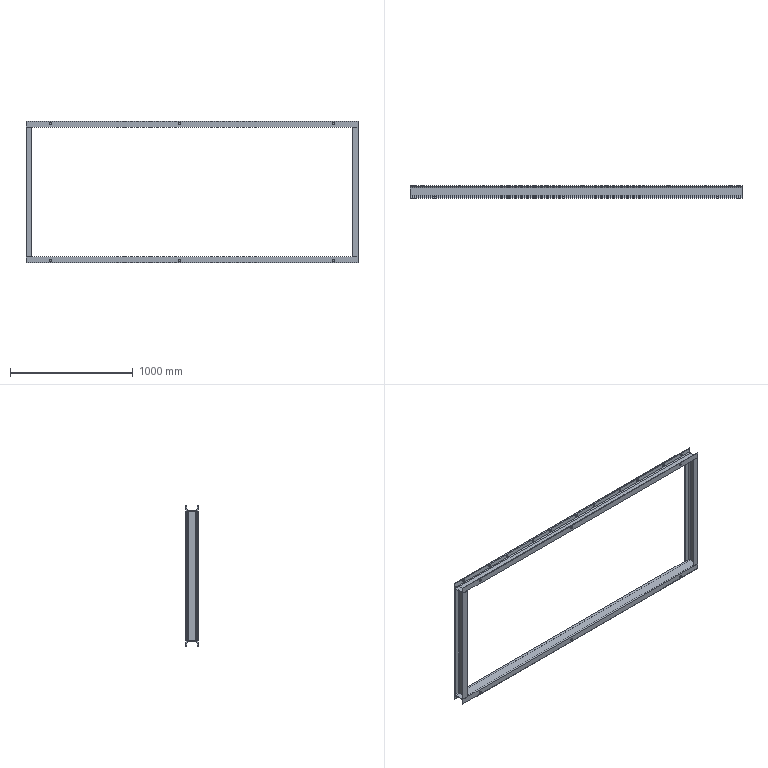Part | STEP file | SW-102-Base3_default<by machining> | 4 solids | 112 faces | box 2705 x 100 x 1155 mm | volume 9416033 mm3 | cylinder 72 | plane 40 | commonest cylinder face diameters 17.29 x44 18 x12 8.5 x8 17 x8